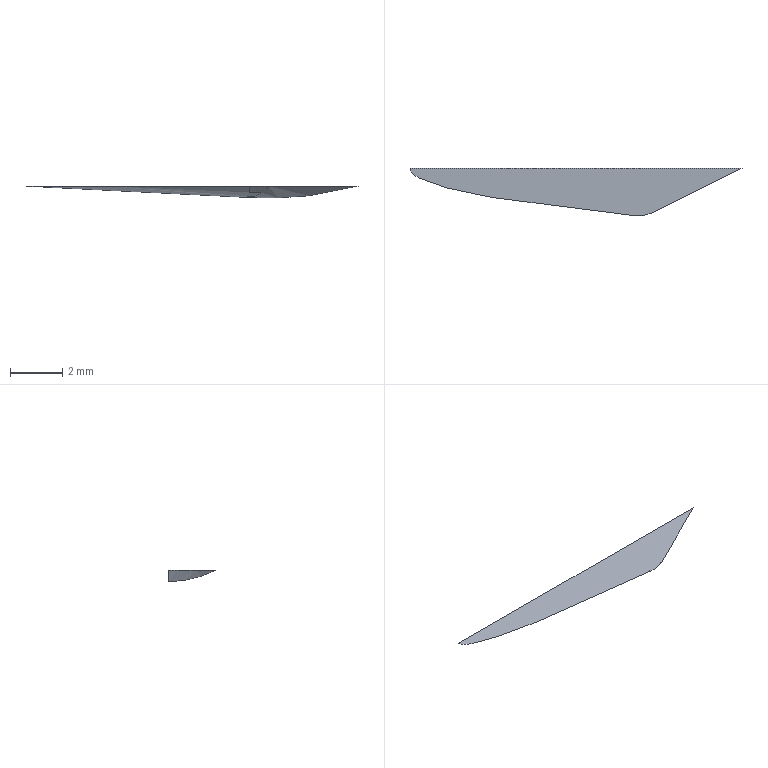Part | STEP file | solid 216 | 1 solid | 5 faces | box 12.653 x 1.816 x 0.4476 mm | volume 2.762 mm3 | plane 2 | spline 2 | cylinder 1 | commonest cylinder face diameters 8 x1